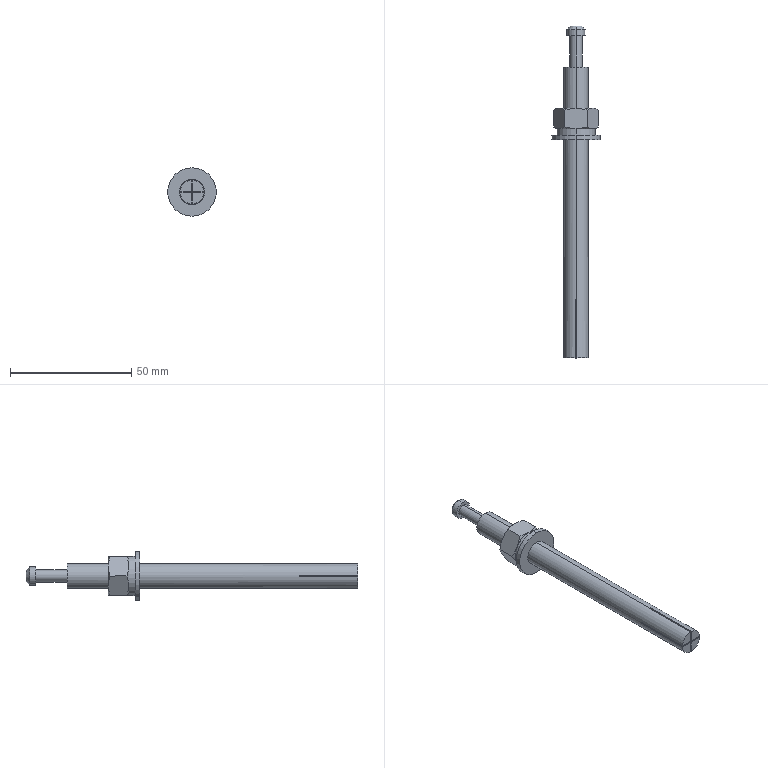Part | STEP file | 5 solids | 64 faces | box 20 x 137 x 20 mm | volume 11527 mm3 | plane 31 | cylinder 18 | cone 15 | commonest cylinder face diameters 10 x4 10.9 x3 16.1 x3 5 x2 7.5 x2 10.5 x2